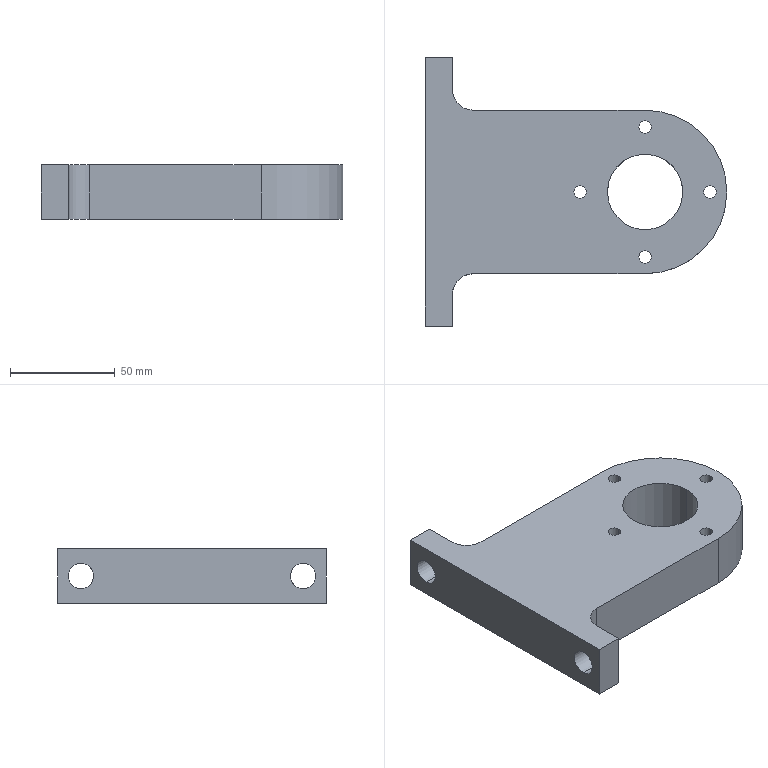Part | NX | features BREP 1 | 1 solid | 26 faces | box 144 x 128 x 26 mm | volume 260725 mm3 | cylinder 17 | plane 9 | commonest cylinder face diameters 6 x8 12 x4 20 x2 36 x2 78 x1
STEP:
#1=CARTESIAN_POINT('',(-92.,53.,7.));
#2=VERTEX_POINT('',#1);
#3=CARTESIAN_POINT('',(-92.,49.,8.528));
#4=VERTEX_POINT('',#3);
#5=CARTESIAN_POINT('',(-92.,53.,13.));
#6=DIRECTION('',(-1.,0.,0.));
#7=DIRECTION('',(0.,0.,1.));
#8=AXIS2_PLACEMENT_3D('',#5,#6,#7);
#9=CIRCLE('',#8,6.);
#10=EDGE_CURVE('',#2,#4,#9,.T.);
#11=ORIENTED_EDGE('',*,*,#10,.F.);
#12=CARTESIAN_POINT('',(-105.,53.,7.));
#13=VERTEX_POINT('',#12);
#14=CARTESIAN_POINT('',(-105.,53.,7.));
#15=DIRECTION('',(-1.,0.,0.));
#16=VECTOR('',#15,1000.);
#17=LINE('',#14,#16);
#18=EDGE_CURVE('',#2,#13,#17,.T.);
#19=ORIENTED_EDGE('',*,*,#18,.T.);
#20=CARTESIAN_POINT('',(-105.,53.,19.));
#21=VERTEX_POINT('',#20);
#22=CARTESIAN_POINT('',(-105.,53.,13.));
#23=DIRECTION('',(-1.,0.,0.));
#24=DIRECTION('',(0.,0.,1.));
#25=AXIS2_PLACEMENT_3D('',#22,#23,#24);
#26=CIRCLE('',#25,6.);
#27=EDGE_CURVE('',#13,#21,#26,.T.);
#28=ORIENTED_EDGE('',*,*,#27,.T.);
#29=CARTESIAN_POINT('',(-92.,53.,19.));
#30=VERTEX_POINT('',#29);
#31=CARTESIAN_POINT('',(-105.,53.,19.));
#32=DIRECTION('',(-1.,0.,0.));
#33=VECTOR('',#32,1000.);
#34=LINE('',#31,#33);
#35=EDGE_CURVE('',#30,#21,#34,.T.);
#36=ORIENTED_EDGE('',*,*,#35,.F.);
#37=CARTESIAN_POINT('',(-92.,49.,17.472));
#38=VERTEX_POINT('',#37);
#39=CARTESIAN_POINT('',(-92.,53.,13.));
#40=DIRECTION('',(-1.,0.,0.));
#41=DIRECTION('',(0.,0.,1.));
#42=AXIS2_PLACEMENT_3D('',#39,#40,#41);
#43=CIRCLE('',#42,6.);
#44=EDGE_CURVE('',#38,#30,#43,.T.);
#45=ORIENTED_EDGE('',*,*,#44,.F.);
#46=CARTESIAN_POINT('',(-92.,49.,8.528));
#47=CARTESIAN_POINT('',(-92.,47.732,9.662));
#48=CARTESIAN_POINT('',(-91.596,46.268,13.001));
#49=CARTESIAN_POINT('',(-92.,47.732,16.338));
#50=CARTESIAN_POINT('',(-92.,49.,17.472));
#51=B_SPLINE_CURVE_WITH_KNOTS('',3,(#46,#47,#48,#49,#50),.UNSPECIFIED.,.F.,.F.,(4,1,4),(0.,0.005027,0.01005),.UNSPECIFIED.);
#52=EDGE_CURVE('',#4,#38,#51,.T.);
#53=ORIENTED_EDGE('',*,*,#52,.F.);
#54=EDGE_LOOP('',(#11,#19,#28,#36,#45,#53));
#55=FACE_BOUND('',#54,.T.);
#56=CARTESIAN_POINT('',(-105.,53.,13.));
#57=DIRECTION('',(-1.,0.,0.));
#58=DIRECTION('',(0.,0.,-1.));
#59=AXIS2_PLACEMENT_3D('',#56,#57,#58);
#60=CYLINDRICAL_SURFACE('',#59,6.);
#61=ADVANCED_FACE('',(#55),#60,.F.);
#62=CARTESIAN_POINT('',(-92.,-53.,7.));
#63=VERTEX_POINT('',#62);
#64=CARTESIAN_POINT('',(-92.,-53.,19.));
#65=VERTEX_POINT('',#64);
#66=CARTESIAN_POINT('',(-92.,-53.,13.));
#67=DIRECTION('',(-1.,0.,0.));
#68=DIRECTION('',(0.,0.,1.));
#69=AXIS2_PLACEMENT_3D('',#66,#67,#68);
#70=CIRCLE('',#69,6.);
#71=EDGE_CURVE('',#63,#65,#70,.T.);
#72=ORIENTED_EDGE('',*,*,#71,.F.);
#73=CARTESIAN_POINT('',(-105.,-53.,7.));
#74=VERTEX_POINT('',#73);
#75=CARTESIAN_POINT('',(-105.,-53.,7.));
#76=DIRECTION('',(-1.,0.,0.));
#77=VECTOR('',#76,1000.);
#78=LINE('',#75,#77);
#79=EDGE_CURVE('',#63,#74,#78,.T.);
#80=ORIENTED_EDGE('',*,*,#79,.T.);
#81=CARTESIAN_POINT('',(-105.,-53.,19.));
#82=VERTEX_POINT('',#81);
#83=CARTESIAN_POINT('',(-105.,-53.,13.));
#84=DIRECTION('',(-1.,0.,0.));
#85=DIRECTION('',(0.,0.,1.));
#86=AXIS2_PLACEMENT_3D('',#83,#84,#85);
#87=CIRCLE('',#86,6.);
#88=EDGE_CURVE('',#74,#82,#87,.T.);
#89=ORIENTED_EDGE('',*,*,#88,.T.);
#90=CARTESIAN_POINT('',(-105.,-53.,19.));
#91=DIRECTION('',(-1.,0.,0.));
#92=VECTOR('',#91,1000.);
#93=LINE('',#90,#92);
#94=EDGE_CURVE('',#65,#82,#93,.T.);
#95=ORIENTED_EDGE('',*,*,#94,.F.);
#96=EDGE_LOOP('',(#72,#80,#89,#95));
#97=FACE_BOUND('',#96,.T.);
#98=CARTESIAN_POINT('',(-105.,-53.,13.));
#99=DIRECTION('',(-1.,0.,0.));
#100=DIRECTION('',(0.,0.,-1.));
#101=AXIS2_PLACEMENT_3D('',#98,#99,#100);
#102=CYLINDRICAL_SURFACE('',#101,6.);
#103=ADVANCED_FACE('',(#97),#102,.F.);
#104=CARTESIAN_POINT('',(-3.,31.,26.));
#105=VERTEX_POINT('',#104);
#106=CARTESIAN_POINT('',(3.,31.,26.));
#107=VERTEX_POINT('',#106);
#108=CARTESIAN_POINT('',(0.,31.,26.));
#109=DIRECTION('',(0.,0.,1.));
#110=DIRECTION('',(1.,0.,0.));
#111=AXIS2_PLACEMENT_3D('',#108,#109,#110);
#112=CIRCLE('',#111,3.);
#113=EDGE_CURVE('',#105,#107,#112,.T.);
#114=ORIENTED_EDGE('',*,*,#113,.T.);
#115=CARTESIAN_POINT('',(3.,31.,0.));
#116=VERTEX_POINT('',#115);
#117=CARTESIAN_POINT('',(3.,31.,26.));
#118=DIRECTION('',(0.,0.,-1.));
#119=VECTOR('',#118,1000.);
#120=LINE('',#117,#119);
#121=EDGE_CURVE('',#116,#107,#120,.F.);
#122=ORIENTED_EDGE('',*,*,#121,.F.);
#123=CARTESIAN_POINT('',(-3.,31.,0.));
#124=VERTEX_POINT('',#123);
#125=CARTESIAN_POINT('',(0.,31.,0.));
#126=DIRECTION('',(0.,0.,1.));
#127=DIRECTION('',(1.,0.,0.));
#128=AXIS2_PLACEMENT_3D('',#125,#126,#127);
#129=CIRCLE('',#128,3.);
#130=EDGE_CURVE('',#124,#116,#129,.T.);
#131=ORIENTED_EDGE('',*,*,#130,.F.);
#132=CARTESIAN_POINT('',(-3.,31.,26.));
#133=DIRECTION('',(0.,0.,-1.));
#134=VECTOR('',#133,1000.);
#135=LINE('',#132,#134);
#136=EDGE_CURVE('',#124,#105,#135,.F.);
#137=ORIENTED_EDGE('',*,*,#136,.T.);
#138=EDGE_LOOP('',(#114,#122,#131,#137));
#139=FACE_BOUND('',#138,.T.);
#140=CARTESIAN_POINT('',(0.,31.,26.));
#141=DIRECTION('',(0.,0.,-1.));
#142=DIRECTION('',(1.,0.,0.));
#143=AXIS2_PLACEMENT_3D('',#140,#141,#142);
#144=CYLINDRICAL_SURFACE('',#143,3.);
#145=ADVANCED_FACE('',(#139),#144,.F.);
#146=CARTESIAN_POINT('',(-34.,0.,26.));
#147=VERTEX_POINT('',#146);
#148=CARTESIAN_POINT('',(-28.,0.,26.));
#149=VERTEX_POINT('',#148);
#150=CARTESIAN_POINT('',(-31.,0.,26.));
#151=DIRECTION('',(0.,0.,1.));
#152=DIRECTION('',(1.,0.,0.));
#153=AXIS2_PLACEMENT_3D('',#150,#151,#152);
#154=CIRCLE('',#153,3.);
#155=EDGE_CURVE('',#147,#149,#154,.T.);
#156=ORIENTED_EDGE('',*,*,#155,.T.);
#157=CARTESIAN_POINT('',(-28.,0.,0.));
#158=VERTEX_POINT('',#157);
#159=CARTESIAN_POINT('',(-28.,0.,26.));
#160=DIRECTION('',(0.,0.,-1.));
#161=VECTOR('',#160,1000.);
#162=LINE('',#159,#161);
#163=EDGE_CURVE('',#158,#149,#162,.F.);
#164=ORIENTED_EDGE('',*,*,#163,.F.);
#165=CARTESIAN_POINT('',(-34.,0.,0.));
#166=VERTEX_POINT('',#165);
#167=CARTESIAN_POINT('',(-31.,0.,0.));
#168=DIRECTION('',(0.,0.,1.));
#169=DIRECTION('',(1.,0.,0.));
#170=AXIS2_PLACEMENT_3D('',#167,#168,#169);
#171=CIRCLE('',#170,3.);
#172=EDGE_CURVE('',#166,#158,#171,.T.);
#173=ORIENTED_EDGE('',*,*,#172,.F.);
#174=CARTESIAN_POINT('',(-34.,0.,26.));
#175=DIRECTION('',(0.,0.,-1.));
#176=VECTOR('',#175,1000.);
#177=LINE('',#174,#176);
#178=EDGE_CURVE('',#166,#147,#177,.F.);
#179=ORIENTED_EDGE('',*,*,#178,.T.);
#180=EDGE_LOOP('',(#156,#164,#173,#179));
#181=FACE_BOUND('',#180,.T.);
#182=CARTESIAN_POINT('',(-31.,0.,26.));
#183=DIRECTION('',(0.,0.,-1.));
#184=DIRECTION('',(1.,0.,0.));
#185=AXIS2_PLACEMENT_3D('',#182,#183,#184);
#186=CYLINDRICAL_SURFACE('',#185,3.);
#187=ADVANCED_FACE('',(#181),#186,.F.);
#188=CARTESIAN_POINT('',(-3.,-31.,26.));
#189=VERTEX_POINT('',#188);
#190=CARTESIAN_POINT('',(3.,-31.,26.));
#191=VERTEX_POINT('',#190);
#192=CARTESIAN_POINT('',(0.,-31.,26.));
#193=DIRECTION('',(0.,0.,1.));
#194=DIRECTION('',(1.,0.,0.));
#195=AXIS2_PLACEMENT_3D('',#192,#193,#194);
#196=CIRCLE('',#195,3.);
#197=EDGE_CURVE('',#189,#191,#196,.T.);
#198=ORIENTED_EDGE('',*,*,#197,.T.);
#199=CARTESIAN_POINT('',(3.,-31.,0.));
#200=VERTEX_POINT('',#199);
#201=CARTESIAN_POINT('',(3.,-31.,26.));
#202=DIRECTION('',(0.,0.,-1.));
#203=VECTOR('',#202,1000.);
#204=LINE('',#201,#203);
#205=EDGE_CURVE('',#200,#191,#204,.F.);
#206=ORIENTED_EDGE('',*,*,#205,.F.);
#207=CARTESIAN_POINT('',(-3.,-31.,0.));
#208=VERTEX_POINT('',#207);
#209=CARTESIAN_POINT('',(0.,-31.,0.));
#210=DIRECTION('',(0.,0.,1.));
#211=DIRECTION('',(1.,0.,0.));
#212=AXIS2_PLACEMENT_3D('',#209,#210,#211);
#213=CIRCLE('',#212,3.);
#214=EDGE_CURVE('',#208,#200,#213,.T.);
#215=ORIENTED_EDGE('',*,*,#214,.F.);
#216=CARTESIAN_POINT('',(-3.,-31.,26.));
#217=DIRECTION('',(0.,0.,-1.));
#218=VECTOR('',#217,1000.);
#219=LINE('',#216,#218);
#220=EDGE_CURVE('',#208,#189,#219,.F.);
#221=ORIENTED_EDGE('',*,*,#220,.T.);
#222=EDGE_LOOP('',(#198,#206,#215,#221));
#223=FACE_BOUND('',#222,.T.);
#224=CARTESIAN_POINT('',(0.,-31.,26.));
#225=DIRECTION('',(0.,0.,-1.));
#226=DIRECTION('',(1.,0.,0.));
#227=AXIS2_PLACEMENT_3D('',#224,#225,#226);
#228=CYLINDRICAL_SURFACE('',#227,3.);
#229=ADVANCED_FACE('',(#223),#228,.F.);
#230=CARTESIAN_POINT('',(28.,0.,26.));
#231=VERTEX_POINT('',#230);
#232=CARTESIAN_POINT('',(34.,0.,26.));
#233=VERTEX_POINT('',#232);
#234=CARTESIAN_POINT('',(31.,0.,26.));
#235=DIRECTION('',(0.,0.,1.));
#236=DIRECTION('',(1.,0.,0.));
#237=AXIS2_PLACEMENT_3D('',#234,#235,#236);
#238=CIRCLE('',#237,3.);
#239=EDGE_CURVE('',#231,#233,#238,.T.);
#240=ORIENTED_EDGE('',*,*,#239,.T.);
#241=CARTESIAN_POINT('',(34.,0.,0.));
#242=VERTEX_POINT('',#241);
#243=CARTESIAN_POINT('',(34.,0.,26.));
#244=DIRECTION('',(0.,0.,-1.));
#245=VECTOR('',#244,1000.);
#246=LINE('',#243,#245);
#247=EDGE_CURVE('',#242,#233,#246,.F.);
#248=ORIENTED_EDGE('',*,*,#247,.F.);
#249=CARTESIAN_POINT('',(28.,0.,0.));
#250=VERTEX_POINT('',#249);
#251=CARTESIAN_POINT('',(31.,0.,0.));
#252=DIRECTION('',(0.,0.,1.));
#253=DIRECTION('',(1.,0.,0.));
#254=AXIS2_PLACEMENT_3D('',#251,#252,#253);
#255=CIRCLE('',#254,3.);
#256=EDGE_CURVE('',#250,#242,#255,.T.);
#257=ORIENTED_EDGE('',*,*,#256,.F.);
#258=CARTESIAN_POINT('',(28.,0.,26.));
#259=DIRECTION('',(0.,0.,-1.));
#260=VECTOR('',#259,1000.);
#261=LINE('',#258,#260);
#262=EDGE_CURVE('',#250,#231,#261,.F.);
#263=ORIENTED_EDGE('',*,*,#262,.T.);
#264=EDGE_LOOP('',(#240,#248,#257,#263));
#265=FACE_BOUND('',#264,.T.);
#266=CARTESIAN_POINT('',(31.,0.,26.));
#267=DIRECTION('',(0.,0.,-1.));
#268=DIRECTION('',(1.,0.,0.));
#269=AXIS2_PLACEMENT_3D('',#266,#267,#268);
#270=CYLINDRICAL_SURFACE('',#269,3.);
#271=ADVANCED_FACE('',(#265),#270,.F.);
#272=CARTESIAN_POINT('',(-18.,0.,26.));
#273=VERTEX_POINT('',#272);
#274=CARTESIAN_POINT('',(18.,0.,26.));
#275=VERTEX_POINT('',#274);
#276=CARTESIAN_POINT('',(0.,0.,26.));
#277=DIRECTION('',(0.,0.,1.));
#278=DIRECTION('',(1.,0.,0.));
#279=AXIS2_PLACEMENT_3D('',#276,#277,#278);
#280=CIRCLE('',#279,18.);
#281=EDGE_CURVE('',#273,#275,#280,.T.);
#282=ORIENTED_EDGE('',*,*,#281,.T.);
#283=CARTESIAN_POINT('',(18.,0.,0.));
#284=VERTEX_POINT('',#283);
#285=CARTESIAN_POINT('',(18.,0.,26.));
#286=DIRECTION('',(0.,0.,-1.));
#287=VECTOR('',#286,1000.);
#288=LINE('',#285,#287);
#289=EDGE_CURVE('',#284,#275,#288,.F.);
#290=ORIENTED_EDGE('',*,*,#289,.F.);
#291=CARTESIAN_POINT('',(-18.,0.,0.));
#292=VERTEX_POINT('',#291);
#293=CARTESIAN_POINT('',(0.,0.,0.));
#294=DIRECTION('',(0.,0.,1.));
#295=DIRECTION('',(1.,0.,0.));
#296=AXIS2_PLACEMENT_3D('',#293,#294,#295);
#297=CIRCLE('',#296,18.);
#298=EDGE_CURVE('',#292,#284,#297,.T.);
#299=ORIENTED_EDGE('',*,*,#298,.F.);
#300=CARTESIAN_POINT('',(-18.,0.,26.));
#301=DIRECTION('',(0.,0.,-1.));
#302=VECTOR('',#301,1000.);
#303=LINE('',#300,#302);
#304=EDGE_CURVE('',#292,#273,#303,.F.);
#305=ORIENTED_EDGE('',*,*,#304,.T.);
#306=EDGE_LOOP('',(#282,#290,#299,#305));
#307=FACE_BOUND('',#306,.T.);
#308=CARTESIAN_POINT('',(0.,0.,26.));
#309=DIRECTION('',(0.,0.,-1.));
#310=DIRECTION('',(1.,0.,0.));
#311=AXIS2_PLACEMENT_3D('',#308,#309,#310);
#312=CYLINDRICAL_SURFACE('',#311,18.);
#313=ADVANCED_FACE('',(#307),#312,.F.);
#314=CARTESIAN_POINT('',(0.,-39.,26.));
#315=VERTEX_POINT('',#314);
#316=CARTESIAN_POINT('',(0.,39.,26.));
#317=VERTEX_POINT('',#316);
#318=CARTESIAN_POINT('',(0.,0.,26.));
#319=DIRECTION('',(0.,0.,1.));
#320=DIRECTION('',(1.,0.,0.));
#321=AXIS2_PLACEMENT_3D('',#318,#319,#320);
#322=CIRCLE('',#321,39.);
#323=EDGE_CURVE('',#315,#317,#322,.T.);
#324=ORIENTED_EDGE('',*,*,#323,.T.);
#325=CARTESIAN_POINT('',(-82.,39.,26.));
#326=VERTEX_POINT('',#325);
#327=CARTESIAN_POINT('',(0.,39.,26.));
#328=DIRECTION('',(-1.,0.,0.));
#329=VECTOR('',#328,1000.);
#330=LINE('',#327,#329);
#331=EDGE_CURVE('',#317,#326,#330,.T.);
#332=ORIENTED_EDGE('',*,*,#331,.T.);
#333=CARTESIAN_POINT('',(-92.,49.,26.));
#334=VERTEX_POINT('',#333);
#335=CARTESIAN_POINT('',(-82.,49.,26.));
#336=DIRECTION('',(0.,0.,-1.));
#337=DIRECTION('',(-1.,0.,0.));
#338=AXIS2_PLACEMENT_3D('',#335,#336,#337);
#339=CIRCLE('',#338,10.);
#340=EDGE_CURVE('',#326,#334,#339,.T.);
#341=ORIENTED_EDGE('',*,*,#340,.T.);
#342=CARTESIAN_POINT('',(-92.,64.,26.));
#343=VERTEX_POINT('',#342);
#344=CARTESIAN_POINT('',(-92.,49.,26.));
#345=DIRECTION('',(0.,1.,0.));
#346=VECTOR('',#345,1000.);
#347=LINE('',#344,#346);
#348=EDGE_CURVE('',#334,#343,#347,.T.);
#349=ORIENTED_EDGE('',*,*,#348,.T.);
#350=CARTESIAN_POINT('',(-105.,64.,26.));
#351=VERTEX_POINT('',#350);
#352=CARTESIAN_POINT('',(-92.,64.,26.));
#353=DIRECTION('',(-1.,0.,0.));
#354=VECTOR('',#353,1000.);
#355=LINE('',#352,#354);
#356=EDGE_CURVE('',#343,#351,#355,.T.);
#357=ORIENTED_EDGE('',*,*,#356,.T.);
#358=CARTESIAN_POINT('',(-105.,-64.,26.));
#359=VERTEX_POINT('',#358);
#360=CARTESIAN_POINT('',(-105.,64.,26.));
#361=DIRECTION('',(0.,-1.,0.));
#362=VECTOR('',#361,1000.);
#363=LINE('',#360,#362);
#364=EDGE_CURVE('',#351,#359,#363,.T.);
#365=ORIENTED_EDGE('',*,*,#364,.T.);
#366=CARTESIAN_POINT('',(-92.,-64.,26.));
#367=VERTEX_POINT('',#366);
#368=CARTESIAN_POINT('',(-92.,-64.,26.));
#369=DIRECTION('',(1.,0.,0.));
#370=VECTOR('',#369,1000.);
#371=LINE('',#368,#370);
#372=EDGE_CURVE('',#359,#367,#371,.T.);
#373=ORIENTED_EDGE('',*,*,#372,.T.);
#374=CARTESIAN_POINT('',(-92.,-49.,26.));
#375=VERTEX_POINT('',#374);
#376=CARTESIAN_POINT('',(-92.,-49.,26.));
#377=DIRECTION('',(0.,1.,0.));
#378=VECTOR('',#377,1000.);
#379=LINE('',#376,#378);
#380=EDGE_CURVE('',#367,#375,#379,.T.);
#381=ORIENTED_EDGE('',*,*,#380,.T.);
#382=CARTESIAN_POINT('',(-82.,-39.,26.));
#383=VERTEX_POINT('',#382);
#384=CARTESIAN_POINT('',(-82.,-49.,26.));
#385=DIRECTION('',(0.,0.,-1.));
#386=DIRECTION('',(1.,0.,0.));
#387=AXIS2_PLACEMENT_3D('',#384,#385,#386);
#388=CIRCLE('',#387,10.);
#389=EDGE_CURVE('',#375,#383,#388,.T.);
#390=ORIENTED_EDGE('',*,*,#389,.T.);
#391=CARTESIAN_POINT('',(0.,-39.,26.));
#392=DIRECTION('',(1.,0.,0.));
#393=VECTOR('',#392,1000.);
#394=LINE('',#391,#393);
#395=EDGE_CURVE('',#383,#315,#394,.T.);
#396=ORIENTED_EDGE('',*,*,#395,.T.);
#397=EDGE_LOOP('',(#324,#332,#341,#349,#357,#365,#373,#381,#390,#396));
#398=FACE_BOUND('',#397,.T.);
#399=ORIENTED_EDGE('',*,*,#155,.F.);
#400=CARTESIAN_POINT('',(-31.,0.,26.));
#401=DIRECTION('',(0.,0.,1.));
#402=DIRECTION('',(1.,0.,0.));
#403=AXIS2_PLACEMENT_3D('',#400,#401,#402);
#404=CIRCLE('',#403,3.);
#405=EDGE_CURVE('',#149,#147,#404,.T.);
#406=ORIENTED_EDGE('',*,*,#405,.F.);
#407=EDGE_LOOP('',(#399,#406));
#408=FACE_BOUND('',#407,.T.);
#409=ORIENTED_EDGE('',*,*,#239,.F.);
#410=CARTESIAN_POINT('',(31.,0.,26.));
#411=DIRECTION('',(0.,0.,1.));
#412=DIRECTION('',(1.,0.,0.));
#413=AXIS2_PLACEMENT_3D('',#410,#411,#412);
#414=CIRCLE('',#413,3.);
#415=EDGE_CURVE('',#233,#231,#414,.T.);
#416=ORIENTED_EDGE('',*,*,#415,.F.);
#417=EDGE_LOOP('',(#409,#416));
#418=FACE_BOUND('',#417,.T.);
#419=ORIENTED_EDGE('',*,*,#281,.F.);
#420=CARTESIAN_POINT('',(0.,0.,26.));
#421=DIRECTION('',(0.,0.,1.));
#422=DIRECTION('',(1.,0.,0.));
#423=AXIS2_PLACEMENT_3D('',#420,#421,#422);
#424=CIRCLE('',#423,18.);
#425=EDGE_CURVE('',#275,#273,#424,.T.);
#426=ORIENTED_EDGE('',*,*,#425,.F.);
#427=EDGE_LOOP('',(#419,#426));
#428=FACE_BOUND('',#427,.T.);
#429=ORIENTED_EDGE('',*,*,#197,.F.);
#430=CARTESIAN_POINT('',(0.,-31.,26.));
#431=DIRECTION('',(0.,0.,1.));
#432=DIRECTION('',(1.,0.,0.));
#433=AXIS2_PLACEMENT_3D('',#430,#431,#432);
#434=CIRCLE('',#433,3.);
#435=EDGE_CURVE('',#191,#189,#434,.T.);
#436=ORIENTED_EDGE('',*,*,#435,.F.);
#437=EDGE_LOOP('',(#429,#436));
#438=FACE_BOUND('',#437,.T.);
#439=ORIENTED_EDGE('',*,*,#113,.F.);
#440=CARTESIAN_POINT('',(0.,31.,26.));
#441=DIRECTION('',(0.,0.,1.));
#442=DIRECTION('',(1.,0.,0.));
#443=AXIS2_PLACEMENT_3D('',#440,#441,#442);
#444=CIRCLE('',#443,3.);
#445=EDGE_CURVE('',#107,#105,#444,.T.);
#446=ORIENTED_EDGE('',*,*,#445,.F.);
#447=EDGE_LOOP('',(#439,#446));
#448=FACE_BOUND('',#447,.T.);
#449=CARTESIAN_POINT('',(0.,0.,26.));
#450=DIRECTION('',(0.,0.,1.));
#451=DIRECTION('',(-1.,0.,0.));
#452=AXIS2_PLACEMENT_3D('',#449,#450,#451);
#453=PLANE('',#452);
#454=ADVANCED_FACE('',(#398,#408,#418,#428,#438,#448),#453,.T.);
#455=CARTESIAN_POINT('',(0.,-39.,0.));
#456=VERTEX_POINT('',#455);
#457=CARTESIAN_POINT('',(0.,39.,0.));
#458=VERTEX_POINT('',#457);
#459=CARTESIAN_POINT('',(0.,0.,0.));
#460=DIRECTION('',(0.,0.,1.));
#461=DIRECTION('',(1.,0.,0.));
#462=AXIS2_PLACEMENT_3D('',#459,#460,#461);
#463=CIRCLE('',#462,39.);
#464=EDGE_CURVE('',#456,#458,#463,.T.);
#465=ORIENTED_EDGE('',*,*,#464,.F.);
#466=CARTESIAN_POINT('',(-82.,-39.,0.));
#467=VERTEX_POINT('',#466);
#468=CARTESIAN_POINT('',(0.,-39.,0.));
#469=DIRECTION('',(1.,0.,0.));
#470=VECTOR('',#469,1000.);
#471=LINE('',#468,#470);
#472=EDGE_CURVE('',#467,#456,#471,.T.);
#473=ORIENTED_EDGE('',*,*,#472,.F.);
#474=CARTESIAN_POINT('',(-92.,-49.,0.));
#475=VERTEX_POINT('',#474);
#476=CARTESIAN_POINT('',(-82.,-49.,0.));
#477=DIRECTION('',(0.,0.,-1.));
#478=DIRECTION('',(1.,0.,0.));
#479=AXIS2_PLACEMENT_3D('',#476,#477,#478);
#480=CIRCLE('',#479,10.);
#481=EDGE_CURVE('',#475,#467,#480,.T.);
#482=ORIENTED_EDGE('',*,*,#481,.F.);
#483=CARTESIAN_POINT('',(-92.,-64.,0.));
#484=VERTEX_POINT('',#483);
#485=CARTESIAN_POINT('',(-92.,-49.,0.));
#486=DIRECTION('',(0.,1.,0.));
#487=VECTOR('',#486,1000.);
#488=LINE('',#485,#487);
#489=EDGE_CURVE('',#484,#475,#488,.T.);
#490=ORIENTED_EDGE('',*,*,#489,.F.);
#491=CARTESIAN_POINT('',(-105.,-64.,0.));
#492=VERTEX_POINT('',#491);
#493=CARTESIAN_POINT('',(-92.,-64.,0.));
#494=DIRECTION('',(1.,0.,0.));
#495=VECTOR('',#494,1000.);
#496=LINE('',#493,#495);
#497=EDGE_CURVE('',#492,#484,#496,.T.);
#498=ORIENTED_EDGE('',*,*,#497,.F.);
#499=CARTESIAN_POINT('',(-105.,64.,0.));
#500=VERTEX_POINT('',#499);
#501=CARTESIAN_POINT('',(-105.,64.,0.));
#502=DIRECTION('',(0.,-1.,0.));
#503=VECTOR('',#502,1000.);
#504=LINE('',#501,#503);
#505=EDGE_CURVE('',#500,#492,#504,.T.);
#506=ORIENTED_EDGE('',*,*,#505,.F.);
#507=CARTESIAN_POINT('',(-92.,64.,0.));
#508=VERTEX_POINT('',#507);
#509=CARTESIAN_POINT('',(-92.,64.,0.));
#510=DIRECTION('',(-1.,0.,0.));
#511=VECTOR('',#510,1000.);
#512=LINE('',#509,#511);
#513=EDGE_CURVE('',#508,#500,#512,.T.);
#514=ORIENTED_EDGE('',*,*,#513,.F.);
#515=CARTESIAN_POINT('',(-92.,49.,0.));
#516=VERTEX_POINT('',#515);
#517=CARTESIAN_POINT('',(-92.,49.,0.));
#518=DIRECTION('',(0.,1.,0.));
#519=VECTOR('',#518,1000.);
#520=LINE('',#517,#519);
#521=EDGE_CURVE('',#516,#508,#520,.T.);
#522=ORIENTED_EDGE('',*,*,#521,.F.);
#523=CARTESIAN_POINT('',(-82.,39.,0.));
#524=VERTEX_POINT('',#523);
#525=CARTESIAN_POINT('',(-82.,49.,0.));
#526=DIRECTION('',(0.,0.,-1.));
#527=DIRECTION('',(-1.,0.,0.));
#528=AXIS2_PLACEMENT_3D('',#525,#526,#527);
#529=CIRCLE('',#528,10.);
#530=EDGE_CURVE('',#524,#516,#529,.T.);
#531=ORIENTED_EDGE('',*,*,#530,.F.);
#532=CARTESIAN_POINT('',(0.,39.,0.));
#533=DIRECTION('',(-1.,0.,0.));
#534=VECTOR('',#533,1000.);
#535=LINE('',#532,#534);
#536=EDGE_CURVE('',#458,#524,#535,.T.);
#537=ORIENTED_EDGE('',*,*,#536,.F.);
#538=EDGE_LOOP('',(#465,#473,#482,#490,#498,#506,#514,#522,#531,#537));
#539=FACE_BOUND('',#538,.T.);
#540=ORIENTED_EDGE('',*,*,#172,.T.);
#541=CARTESIAN_POINT('',(-31.,0.,0.));
#542=DIRECTION('',(0.,0.,1.));
#543=DIRECTION('',(1.,0.,0.));
#544=AXIS2_PLACEMENT_3D('',#541,#542,#543);
#545=CIRCLE('',#544,3.);
#546=EDGE_CURVE('',#158,#166,#545,.T.);
#547=ORIENTED_EDGE('',*,*,#546,.T.);
#548=EDGE_LOOP('',(#540,#547));
#549=FACE_BOUND('',#548,.T.);
#550=ORIENTED_EDGE('',*,*,#256,.T.);
#551=CARTESIAN_POINT('',(31.,0.,0.));
#552=DIRECTION('',(0.,0.,1.));
#553=DIRECTION('',(1.,0.,0.));
#554=AXIS2_PLACEMENT_3D('',#551,#552,#553);
#555=CIRCLE('',#554,3.);
#556=EDGE_CURVE('',#242,#250,#555,.T.);
#557=ORIENTED_EDGE('',*,*,#556,.T.);
#558=EDGE_LOOP('',(#550,#557));
#559=FACE_BOUND('',#558,.T.);
#560=ORIENTED_EDGE('',*,*,#298,.T.);
#561=CARTESIAN_POINT('',(0.,0.,0.));
#562=DIRECTION('',(0.,0.,1.));
#563=DIRECTION('',(1.,0.,0.));
#564=AXIS2_PLACEMENT_3D('',#561,#562,#563);
#565=CIRCLE('',#564,18.);
#566=EDGE_CURVE('',#284,#292,#565,.T.);
#567=ORIENTED_EDGE('',*,*,#566,.T.);
#568=EDGE_LOOP('',(#560,#567));
#569=FACE_BOUND('',#568,.T.);
#570=ORIENTED_EDGE('',*,*,#214,.T.);
#571=CARTESIAN_POINT('',(0.,-31.,0.));
#572=DIRECTION('',(0.,0.,1.));
#573=DIRECTION('',(1.,0.,0.));
#574=AXIS2_PLACEMENT_3D('',#571,#572,#573);
#575=CIRCLE('',#574,3.);
#576=EDGE_CURVE('',#200,#208,#575,.T.);
#577=ORIENTED_EDGE('',*,*,#576,.T.);
#578=EDGE_LOOP('',(#570,#577));
#579=FACE_BOUND('',#578,.T.);
#580=ORIENTED_EDGE('',*,*,#130,.T.);
#581=CARTESIAN_POINT('',(0.,31.,0.));
#582=DIRECTION('',(0.,0.,1.));
#583=DIRECTION('',(1.,0.,0.));
#584=AXIS2_PLACEMENT_3D('',#581,#582,#583);
#585=CIRCLE('',#584,3.);
#586=EDGE_CURVE('',#116,#124,#585,.T.);
#587=ORIENTED_EDGE('',*,*,#586,.T.);
#588=EDGE_LOOP('',(#580,#587));
#589=FACE_BOUND('',#588,.T.);
#590=CARTESIAN_POINT('',(0.,0.,0.));
#591=DIRECTION('',(0.,0.,1.));
#592=DIRECTION('',(-1.,0.,0.));
#593=AXIS2_PLACEMENT_3D('',#590,#591,#592);
#594=PLANE('',#593);
#595=ADVANCED_FACE('',(#539,#549,#559,#569,#579,#589),#594,.F.);
#596=ORIENTED_EDGE('',*,*,#464,.T.);
#597=CARTESIAN_POINT('',(0.,39.,26.));
#598=DIRECTION('',(0.,0.,-1.));
#599=VECTOR('',#598,1000.);
#600=LINE('',#597,#599);
#601=EDGE_CURVE('',#317,#458,#600,.T.);
#602=ORIENTED_EDGE('',*,*,#601,.F.);
#603=ORIENTED_EDGE('',*,*,#323,.F.);
#604=CARTESIAN_POINT('',(0.,-39.,26.));
#605=DIRECTION('',(0.,0.,-1.));
#606=VECTOR('',#605,1000.);
#607=LINE('',#604,#606);
#608=EDGE_CURVE('',#315,#456,#607,.T.);
#609=ORIENTED_EDGE('',*,*,#608,.T.);
#610=EDGE_LOOP('',(#596,#602,#603,#609));
#611=FACE_BOUND('',#610,.T.);
#612=CARTESIAN_POINT('',(0.,0.,26.));
#613=DIRECTION('',(0.,0.,-1.));
#614=DIRECTION('',(1.,0.,0.));
#615=AXIS2_PLACEMENT_3D('',#612,#613,#614);
#616=CYLINDRICAL_SURFACE('',#615,39.);
#617=ADVANCED_FACE('',(#611),#616,.T.);
#618=ORIENTED_EDGE('',*,*,#536,.T.);
#619=CARTESIAN_POINT('',(-82.,39.,26.));
#620=DIRECTION('',(0.,0.,-1.));
#621=VECTOR('',#620,1000.);
#622=LINE('',#619,#621);
#623=EDGE_CURVE('',#326,#524,#622,.T.);
#624=ORIENTED_EDGE('',*,*,#623,.F.);
#625=ORIENTED_EDGE('',*,*,#331,.F.);
#626=ORIENTED_EDGE('',*,*,#601,.T.);
#627=EDGE_LOOP('',(#618,#624,#625,#626));
#628=FACE_BOUND('',#627,.T.);
#629=CARTESIAN_POINT('',(0.,39.,26.));
#630=DIRECTION('',(0.,-1.,0.));
#631=DIRECTION('',(0.,0.,1.));
#632=AXIS2_PLACEMENT_3D('',#629,#630,#631);
#633=PLANE('',#632);
#634=ADVANCED_FACE('',(#628),#633,.F.);
#635=CARTESIAN_POINT('',(-92.,49.,26.));
#636=DIRECTION('',(0.,0.,-1.));
#637=VECTOR('',#636,1000.);
#638=LINE('',#635,#637);
#639=EDGE_CURVE('',#4,#516,#638,.T.);
#640=ORIENTED_EDGE('',*,*,#639,.F.);
#641=ORIENTED_EDGE('',*,*,#52,.T.);
#642=CARTESIAN_POINT('',(-92.,49.,26.));
#643=DIRECTION('',(0.,0.,-1.));
#644=VECTOR('',#643,1000.);
#645=LINE('',#642,#644);
#646=EDGE_CURVE('',#334,#38,#645,.T.);
#647=ORIENTED_EDGE('',*,*,#646,.F.);
#648=ORIENTED_EDGE('',*,*,#340,.F.);
#649=ORIENTED_EDGE('',*,*,#623,.T.);
#650=ORIENTED_EDGE('',*,*,#530,.T.);
#651=EDGE_LOOP('',(#640,#641,#647,#648,#649,#650));
#652=FACE_BOUND('',#651,.T.);
#653=CARTESIAN_POINT('',(-82.,49.,26.));
#654=DIRECTION('',(0.,0.,-1.));
#655=DIRECTION('',(1.,0.,0.));
#656=AXIS2_PLACEMENT_3D('',#653,#654,#655);
#657=CYLINDRICAL_SURFACE('',#656,10.);
#658=ADVANCED_FACE('',(#652),#657,.F.);
#659=ORIENTED_EDGE('',*,*,#646,.T.);
#660=ORIENTED_EDGE('',*,*,#44,.T.);
#661=CARTESIAN_POINT('',(-92.,53.,13.));
#662=DIRECTION('',(-1.,0.,0.));
#663=DIRECTION('',(0.,0.,1.));
#664=AXIS2_PLACEMENT_3D('',#661,#662,#663);
#665=CIRCLE('',#664,6.);
#666=EDGE_CURVE('',#30,#2,#665,.T.);
#667=ORIENTED_EDGE('',*,*,#666,.T.);
#668=ORIENTED_EDGE('',*,*,#10,.T.);
#669=ORIENTED_EDGE('',*,*,#639,.T.);
#670=ORIENTED_EDGE('',*,*,#521,.T.);
#671=CARTESIAN_POINT('',(-92.,64.,26.));
#672=DIRECTION('',(0.,0.,-1.));
#673=VECTOR('',#672,1000.);
#674=LINE('',#671,#673);
#675=EDGE_CURVE('',#343,#508,#674,.T.);
#676=ORIENTED_EDGE('',*,*,#675,.F.);
#677=ORIENTED_EDGE('',*,*,#348,.F.);
#678=EDGE_LOOP('',(#659,#660,#667,#668,#669,#670,#676,#677));
#679=FACE_BOUND('',#678,.T.);
#680=CARTESIAN_POINT('',(-92.,49.,26.));
#681=DIRECTION('',(-1.,0.,0.));
#682=DIRECTION('',(0.,0.,-1.));
#683=AXIS2_PLACEMENT_3D('',#680,#681,#682);
#684=PLANE('',#683);
#685=ADVANCED_FACE('',(#679),#684,.F.);
#686=ORIENTED_EDGE('',*,*,#513,.T.);
#687=CARTESIAN_POINT('',(-105.,64.,26.));
#688=DIRECTION('',(0.,0.,-1.));
#689=VECTOR('',#688,1000.);
#690=LINE('',#687,#689);
#691=EDGE_CURVE('',#351,#500,#690,.T.);
#692=ORIENTED_EDGE('',*,*,#691,.F.);
#693=ORIENTED_EDGE('',*,*,#356,.F.);
#694=ORIENTED_EDGE('',*,*,#675,.T.);
#695=EDGE_LOOP('',(#686,#692,#693,#694));
#696=FACE_BOUND('',#695,.T.);
#697=CARTESIAN_POINT('',(-92.,64.,26.));
#698=DIRECTION('',(0.,-1.,0.));
#699=DIRECTION('',(0.,0.,1.));
#700=AXIS2_PLACEMENT_3D('',#697,#698,#699);
#701=PLANE('',#700);
#702=ADVANCED_FACE('',(#696),#701,.F.);
#703=ORIENTED_EDGE('',*,*,#505,.T.);
#704=CARTESIAN_POINT('',(-105.,-64.,26.));
#705=DIRECTION('',(0.,0.,-1.));
#706=VECTOR('',#705,1000.);
#707=LINE('',#704,#706);
#708=EDGE_CURVE('',#359,#492,#707,.T.);
#709=ORIENTED_EDGE('',*,*,#708,.F.);
#710=ORIENTED_EDGE('',*,*,#364,.F.);
#711=ORIENTED_EDGE('',*,*,#691,.T.);
#712=EDGE_LOOP('',(#703,#709,#710,#711));
#713=FACE_BOUND('',#712,.T.);
#714=CARTESIAN_POINT('',(-105.,53.,13.));
#715=DIRECTION('',(-1.,0.,0.));
#716=DIRECTION('',(0.,0.,1.));
#717=AXIS2_PLACEMENT_3D('',#714,#715,#716);
#718=CIRCLE('',#717,6.);
#719=EDGE_CURVE('',#21,#13,#718,.T.);
#720=ORIENTED_EDGE('',*,*,#719,.F.);
#721=ORIENTED_EDGE('',*,*,#27,.F.);
#722=EDGE_LOOP('',(#720,#721));
#723=FACE_BOUND('',#722,.T.);
#724=CARTESIAN_POINT('',(-105.,-53.,13.));
#725=DIRECTION('',(-1.,0.,0.));
#726=DIRECTION('',(0.,0.,1.));
#727=AXIS2_PLACEMENT_3D('',#724,#725,#726);
#728=CIRCLE('',#727,6.);
#729=EDGE_CURVE('',#82,#74,#728,.T.);
#730=ORIENTED_EDGE('',*,*,#729,.F.);
#731=ORIENTED_EDGE('',*,*,#88,.F.);
#732=EDGE_LOOP('',(#730,#731));
#733=FACE_BOUND('',#732,.T.);
#734=CARTESIAN_POINT('',(-105.,64.,26.));
#735=DIRECTION('',(1.,0.,0.));
#736=DIRECTION('',(0.,-1.,0.));
#737=AXIS2_PLACEMENT_3D('',#734,#735,#736);
#738=PLANE('',#737);
#739=ADVANCED_FACE('',(#713,#723,#733),#738,.F.);
#740=ORIENTED_EDGE('',*,*,#497,.T.);
#741=CARTESIAN_POINT('',(-92.,-64.,26.));
#742=DIRECTION('',(0.,0.,-1.));
#743=VECTOR('',#742,1000.);
#744=LINE('',#741,#743);
#745=EDGE_CURVE('',#367,#484,#744,.T.);
#746=ORIENTED_EDGE('',*,*,#745,.F.);
#747=ORIENTED_EDGE('',*,*,#372,.F.);
#748=ORIENTED_EDGE('',*,*,#708,.T.);
#749=EDGE_LOOP('',(#740,#746,#747,#748));
#750=FACE_BOUND('',#749,.T.);
#751=CARTESIAN_POINT('',(-92.,-64.,26.));
#752=DIRECTION('',(0.,1.,0.));
#753=DIRECTION('',(-1.,0.,0.));
#754=AXIS2_PLACEMENT_3D('',#751,#752,#753);
#755=PLANE('',#754);
#756=ADVANCED_FACE('',(#750),#755,.F.);
#757=CARTESIAN_POINT('',(-92.,-49.,8.528));
#758=VERTEX_POINT('',#757);
#759=CARTESIAN_POINT('',(-92.,-49.,26.));
#760=DIRECTION('',(0.,0.,-1.));
#761=VECTOR('',#760,1000.);
#762=LINE('',#759,#761);
#763=EDGE_CURVE('',#758,#475,#762,.T.);
#764=ORIENTED_EDGE('',*,*,#763,.F.);
#765=CARTESIAN_POINT('',(-92.,-53.,13.));
#766=DIRECTION('',(-1.,0.,0.));
#767=DIRECTION('',(0.,0.,1.));
#768=AXIS2_PLACEMENT_3D('',#765,#766,#767);
#769=CIRCLE('',#768,6.);
#770=EDGE_CURVE('',#758,#63,#769,.T.);
#771=ORIENTED_EDGE('',*,*,#770,.T.);
#772=ORIENTED_EDGE('',*,*,#71,.T.);
#773=CARTESIAN_POINT('',(-92.,-49.,17.472));
#774=VERTEX_POINT('',#773);
#775=CARTESIAN_POINT('',(-92.,-53.,13.));
#776=DIRECTION('',(-1.,0.,0.));
#777=DIRECTION('',(0.,0.,1.));
#778=AXIS2_PLACEMENT_3D('',#775,#776,#777);
#779=CIRCLE('',#778,6.);
#780=EDGE_CURVE('',#65,#774,#779,.T.);
#781=ORIENTED_EDGE('',*,*,#780,.T.);
#782=CARTESIAN_POINT('',(-92.,-49.,26.));
#783=DIRECTION('',(0.,0.,-1.));
#784=VECTOR('',#783,1000.);
#785=LINE('',#782,#784);
#786=EDGE_CURVE('',#375,#774,#785,.T.);
#787=ORIENTED_EDGE('',*,*,#786,.F.);
#788=ORIENTED_EDGE('',*,*,#380,.F.);
#789=ORIENTED_EDGE('',*,*,#745,.T.);
#790=ORIENTED_EDGE('',*,*,#489,.T.);
#791=EDGE_LOOP('',(#764,#771,#772,#781,#787,#788,#789,#790));
#792=FACE_BOUND('',#791,.T.);
#793=CARTESIAN_POINT('',(-92.,-49.,26.));
#794=DIRECTION('',(-1.,0.,0.));
#795=DIRECTION('',(0.,0.,-1.));
#796=AXIS2_PLACEMENT_3D('',#793,#794,#795);
#797=PLANE('',#796);
#798=ADVANCED_FACE('',(#792),#797,.F.);
#799=ORIENTED_EDGE('',*,*,#786,.T.);
#800=CARTESIAN_POINT('',(-92.,-49.,17.472));
#801=CARTESIAN_POINT('',(-92.,-47.732,16.338));
#802=CARTESIAN_POINT('',(-91.596,-46.268,12.999));
#803=CARTESIAN_POINT('',(-92.,-47.732,9.662));
#804=CARTESIAN_POINT('',(-92.,-49.,8.528));
#805=B_SPLINE_CURVE_WITH_KNOTS('',3,(#800,#801,#802,#803,#804),.UNSPECIFIED.,.F.,.F.,(4,1,4),(0.,0.005027,0.01005),.UNSPECIFIED.);
#806=EDGE_CURVE('',#774,#758,#805,.T.);
#807=ORIENTED_EDGE('',*,*,#806,.T.);
#808=ORIENTED_EDGE('',*,*,#763,.T.);
#809=ORIENTED_EDGE('',*,*,#481,.T.);
#810=CARTESIAN_POINT('',(-82.,-39.,26.));
#811=DIRECTION('',(0.,0.,-1.));
#812=VECTOR('',#811,1000.);
#813=LINE('',#810,#812);
#814=EDGE_CURVE('',#383,#467,#813,.T.);
#815=ORIENTED_EDGE('',*,*,#814,.F.);
#816=ORIENTED_EDGE('',*,*,#389,.F.);
#817=EDGE_LOOP('',(#799,#807,#808,#809,#815,#816));
#818=FACE_BOUND('',#817,.T.);
#819=CARTESIAN_POINT('',(-82.,-49.,26.));
#820=DIRECTION('',(0.,0.,-1.));
#821=DIRECTION('',(1.,0.,0.));
#822=AXIS2_PLACEMENT_3D('',#819,#820,#821);
#823=CYLINDRICAL_SURFACE('',#822,10.);
#824=ADVANCED_FACE('',(#818),#823,.F.);
#825=ORIENTED_EDGE('',*,*,#472,.T.);
#826=ORIENTED_EDGE('',*,*,#608,.F.);
#827=ORIENTED_EDGE('',*,*,#395,.F.);
#828=ORIENTED_EDGE('',*,*,#814,.T.);
#829=EDGE_LOOP('',(#825,#826,#827,#828));
#830=FACE_BOUND('',#829,.T.);
#831=CARTESIAN_POINT('',(0.,-39.,26.));
#832=DIRECTION('',(0.,1.,0.));
#833=DIRECTION('',(-1.,0.,0.));
#834=AXIS2_PLACEMENT_3D('',#831,#832,#833);
#835=PLANE('',#834);
#836=ADVANCED_FACE('',(#830),#835,.F.);
#837=ORIENTED_EDGE('',*,*,#289,.T.);
#838=ORIENTED_EDGE('',*,*,#425,.T.);
#839=ORIENTED_EDGE('',*,*,#304,.F.);
#840=ORIENTED_EDGE('',*,*,#566,.F.);
#841=EDGE_LOOP('',(#837,#838,#839,#840));
#842=FACE_BOUND('',#841,.T.);
#843=CARTESIAN_POINT('',(0.,0.,26.));
#844=DIRECTION('',(0.,0.,-1.));
#845=DIRECTION('',(1.,0.,0.));
#846=AXIS2_PLACEMENT_3D('',#843,#844,#845);
#847=CYLINDRICAL_SURFACE('',#846,18.);
#848=ADVANCED_FACE('',(#842),#847,.F.);
#849=ORIENTED_EDGE('',*,*,#247,.T.);
#850=ORIENTED_EDGE('',*,*,#415,.T.);
#851=ORIENTED_EDGE('',*,*,#262,.F.);
#852=ORIENTED_EDGE('',*,*,#556,.F.);
#853=EDGE_LOOP('',(#849,#850,#851,#852));
#854=FACE_BOUND('',#853,.T.);
#855=CARTESIAN_POINT('',(31.,0.,26.));
#856=DIRECTION('',(0.,0.,-1.));
#857=DIRECTION('',(1.,0.,0.));
#858=AXIS2_PLACEMENT_3D('',#855,#856,#857);
#859=CYLINDRICAL_SURFACE('',#858,3.);
#860=ADVANCED_FACE('',(#854),#859,.F.);
#861=ORIENTED_EDGE('',*,*,#205,.T.);
#862=ORIENTED_EDGE('',*,*,#435,.T.);
#863=ORIENTED_EDGE('',*,*,#220,.F.);
#864=ORIENTED_EDGE('',*,*,#576,.F.);
#865=EDGE_LOOP('',(#861,#862,#863,#864));
#866=FACE_BOUND('',#865,.T.);
#867=CARTESIAN_POINT('',(0.,-31.,26.));
#868=DIRECTION('',(0.,0.,-1.));
#869=DIRECTION('',(1.,0.,0.));
#870=AXIS2_PLACEMENT_3D('',#867,#868,#869);
#871=CYLINDRICAL_SURFACE('',#870,3.);
#872=ADVANCED_FACE('',(#866),#871,.F.);
#873=ORIENTED_EDGE('',*,*,#163,.T.);
#874=ORIENTED_EDGE('',*,*,#405,.T.);
#875=ORIENTED_EDGE('',*,*,#178,.F.);
#876=ORIENTED_EDGE('',*,*,#546,.F.);
#877=EDGE_LOOP('',(#873,#874,#875,#876));
#878=FACE_BOUND('',#877,.T.);
#879=CARTESIAN_POINT('',(-31.,0.,26.));
#880=DIRECTION('',(0.,0.,-1.));
#881=DIRECTION('',(1.,0.,0.));
#882=AXIS2_PLACEMENT_3D('',#879,#880,#881);
#883=CYLINDRICAL_SURFACE('',#882,3.);
#884=ADVANCED_FACE('',(#878),#883,.F.);
#885=ORIENTED_EDGE('',*,*,#121,.T.);
#886=ORIENTED_EDGE('',*,*,#445,.T.);
#887=ORIENTED_EDGE('',*,*,#136,.F.);
#888=ORIENTED_EDGE('',*,*,#586,.F.);
#889=EDGE_LOOP('',(#885,#886,#887,#888));
#890=FACE_BOUND('',#889,.T.);
#891=CARTESIAN_POINT('',(0.,31.,26.));
#892=DIRECTION('',(0.,0.,-1.));
#893=DIRECTION('',(1.,0.,0.));
#894=AXIS2_PLACEMENT_3D('',#891,#892,#893);
#895=CYLINDRICAL_SURFACE('',#894,3.);
#896=ADVANCED_FACE('',(#890),#895,.F.);
#897=ORIENTED_EDGE('',*,*,#79,.F.);
#898=ORIENTED_EDGE('',*,*,#770,.F.);
#899=ORIENTED_EDGE('',*,*,#806,.F.);
#900=ORIENTED_EDGE('',*,*,#780,.F.);
#901=ORIENTED_EDGE('',*,*,#94,.T.);
#902=ORIENTED_EDGE('',*,*,#729,.T.);
#903=EDGE_LOOP('',(#897,#898,#899,#900,#901,#902));
#904=FACE_BOUND('',#903,.T.);
#905=CARTESIAN_POINT('',(-105.,-53.,13.));
#906=DIRECTION('',(-1.,0.,0.));
#907=DIRECTION('',(0.,0.,-1.));
#908=AXIS2_PLACEMENT_3D('',#905,#906,#907);
#909=CYLINDRICAL_SURFACE('',#908,6.);
#910=ADVANCED_FACE('',(#904),#909,.F.);
#911=ORIENTED_EDGE('',*,*,#18,.F.);
#912=ORIENTED_EDGE('',*,*,#666,.F.);
#913=ORIENTED_EDGE('',*,*,#35,.T.);
#914=ORIENTED_EDGE('',*,*,#719,.T.);
#915=EDGE_LOOP('',(#911,#912,#913,#914));
#916=FACE_BOUND('',#915,.T.);
#917=CARTESIAN_POINT('',(-105.,53.,13.));
#918=DIRECTION('',(-1.,0.,0.));
#919=DIRECTION('',(0.,0.,-1.));
#920=AXIS2_PLACEMENT_3D('',#917,#918,#919);
#921=CYLINDRICAL_SURFACE('',#920,6.);
#922=ADVANCED_FACE('',(#916),#921,.F.);
#923=CLOSED_SHELL('',(#61,#103,#145,#187,#229,#271,#313,#454,#595,#617,#634,#658,#685,#702,#739,#756,#798,#824,#836,#848,#860,#872,#884,#896,#910,#922));
#924=MANIFOLD_SOLID_BREP('',#923);
#925=(LENGTH_UNIT()NAMED_UNIT(*)SI_UNIT(.MILLI.,.METRE.));
#926=UNCERTAINTY_MEASURE_WITH_UNIT(LENGTH_MEASURE(0.0508),#925,'','');
#927=(NAMED_UNIT(*)PLANE_ANGLE_UNIT()SI_UNIT($,.RADIAN.));
#928=(NAMED_UNIT(*)SI_UNIT($,.STERADIAN.)SOLID_ANGLE_UNIT());
#929=(GEOMETRIC_REPRESENTATION_CONTEXT(3)GLOBAL_UNCERTAINTY_ASSIGNED_CONTEXT((#926))GLOBAL_UNIT_ASSIGNED_CONTEXT((#925,#927,#928))REPRESENTATION_CONTEXT('',''));
#930=ADVANCED_BREP_SHAPE_REPRESENTATION('',(#924),#929);